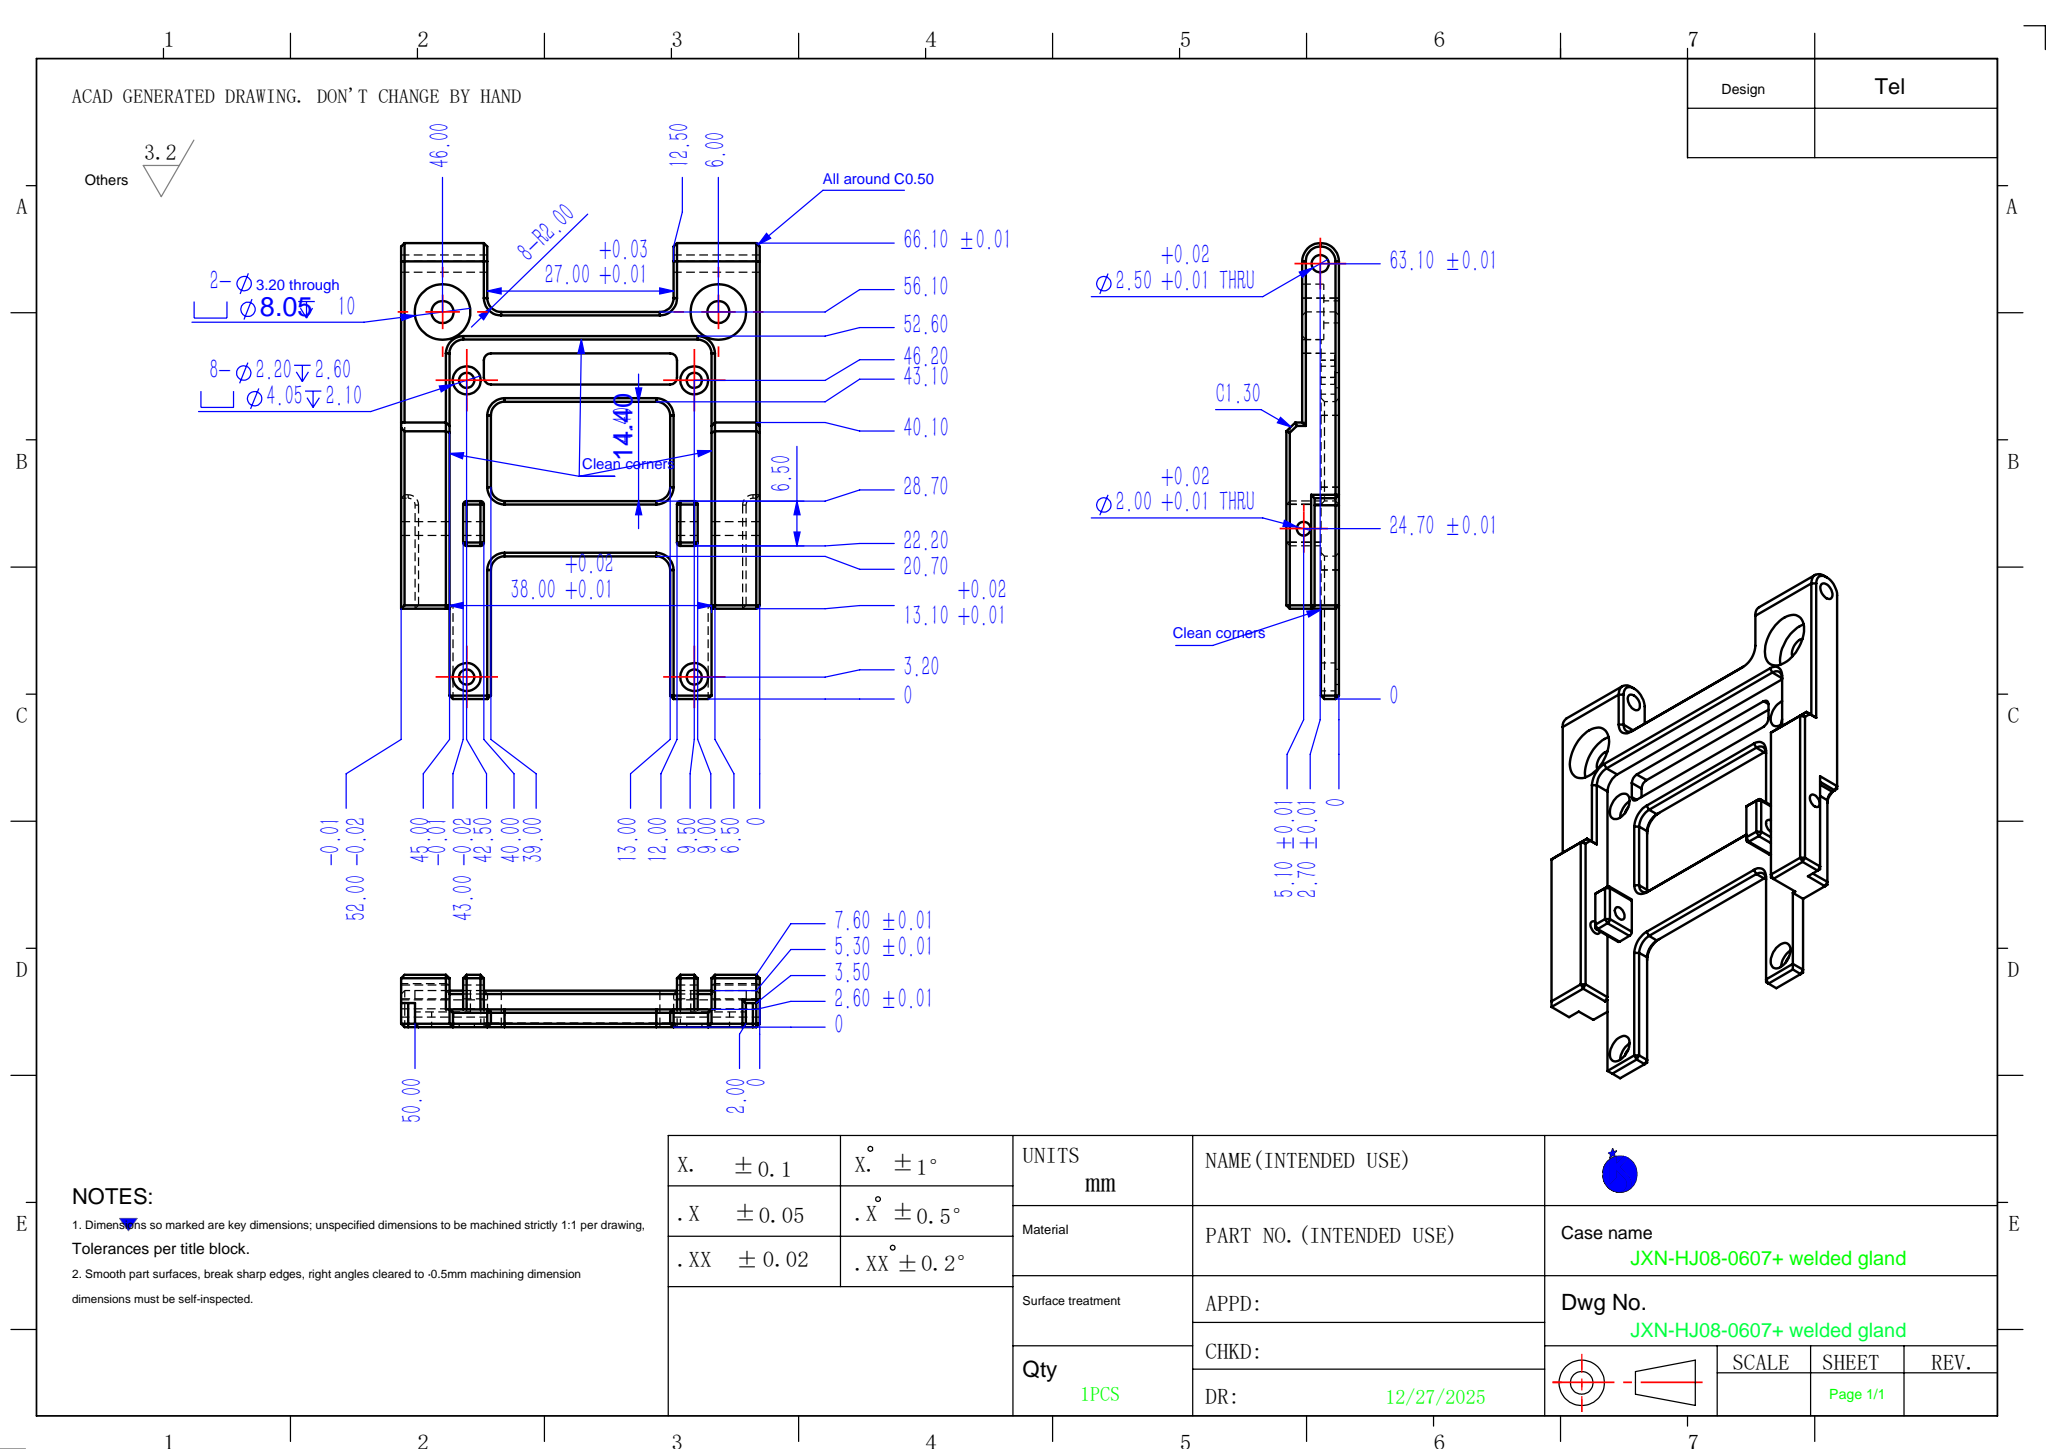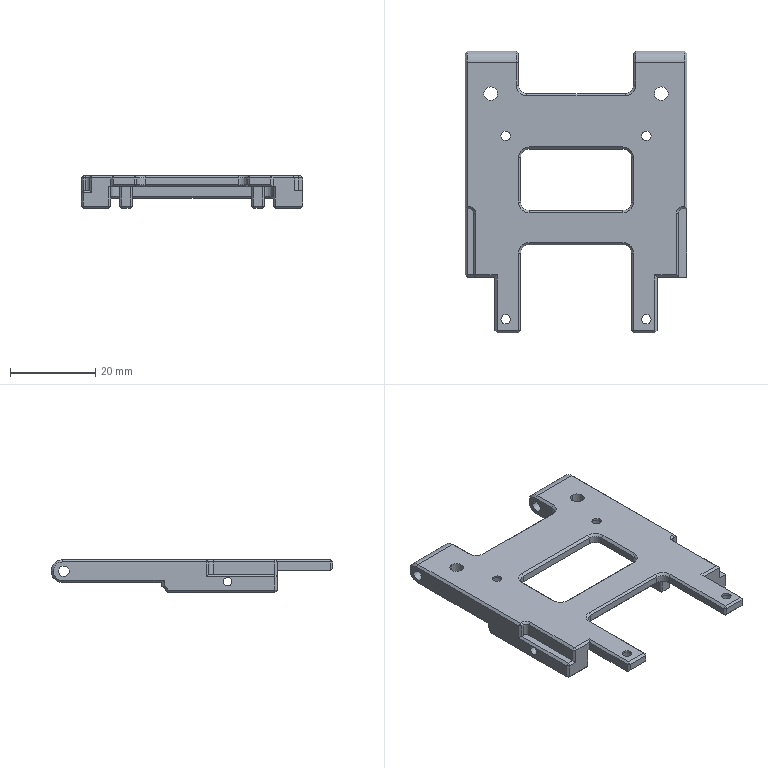Part | SolidWorks | features ICE 16, Fillet 6, Chamfer 2, MoveFace 2, Cut 1, DelFace 1, Extrusion 1 | 1 solid | 239 faces | box 52 x 66.1 x 7.6 mm | volume 7864 mm3 | plane 139 | cylinder 64 | cone 36 | commonest cylinder face diameters 2 x14 4 x10 1 x8 2.2 x8 4.05 x8 2.5 x4